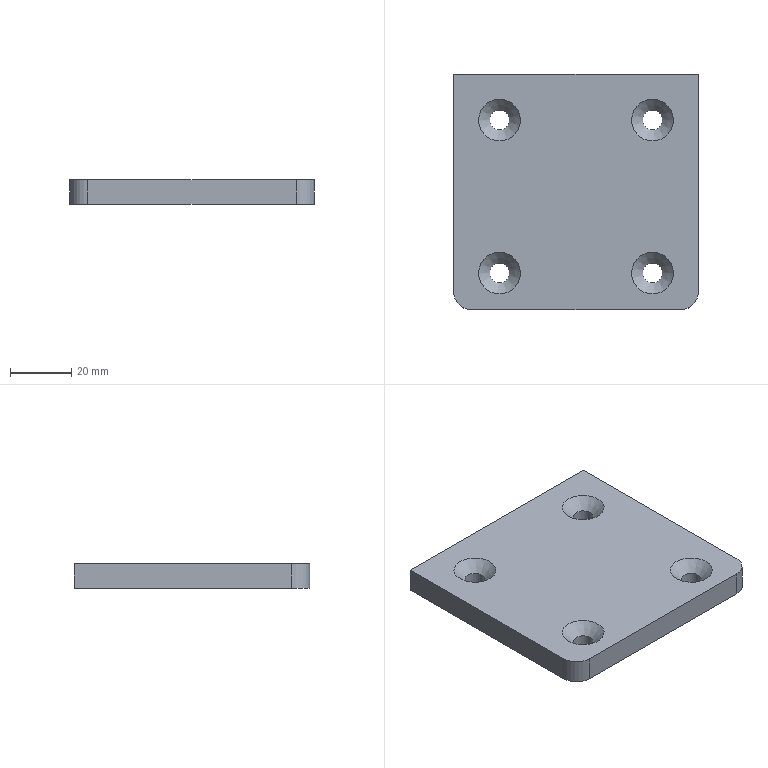Part | STEP file | solid 61 | 1 solid | 16 faces | box 80 x 77 x 8 mm | volume 47370 mm3 | plane 6 | cylinder 6 | cone 4 | commonest cylinder face diameters 6.5 x4 12 x2